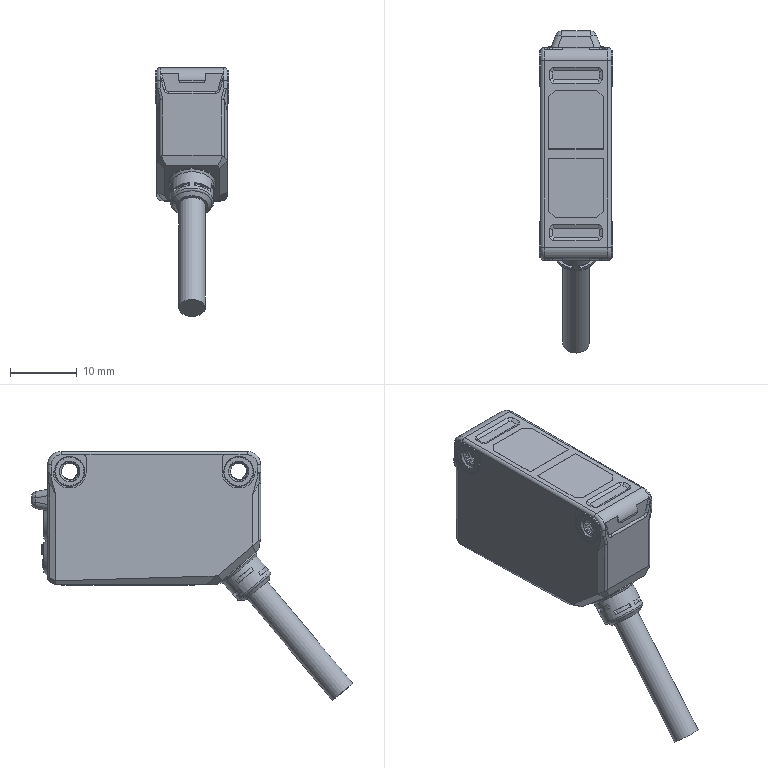Part | STEP file | ROTATION MC_NEW VER-0610_507 | 1 solid | 638 faces | box 11 x 48.371 x 37.42 mm | volume 6844 mm3 | plane 287 | cylinder 277 | spline 40 | torus 17 | cone 13 | sphere 4 | commonest cylinder face diameters 0.45 x128 2.5 x42 1 x31 2 x12 3.1 x10 0.4 x8